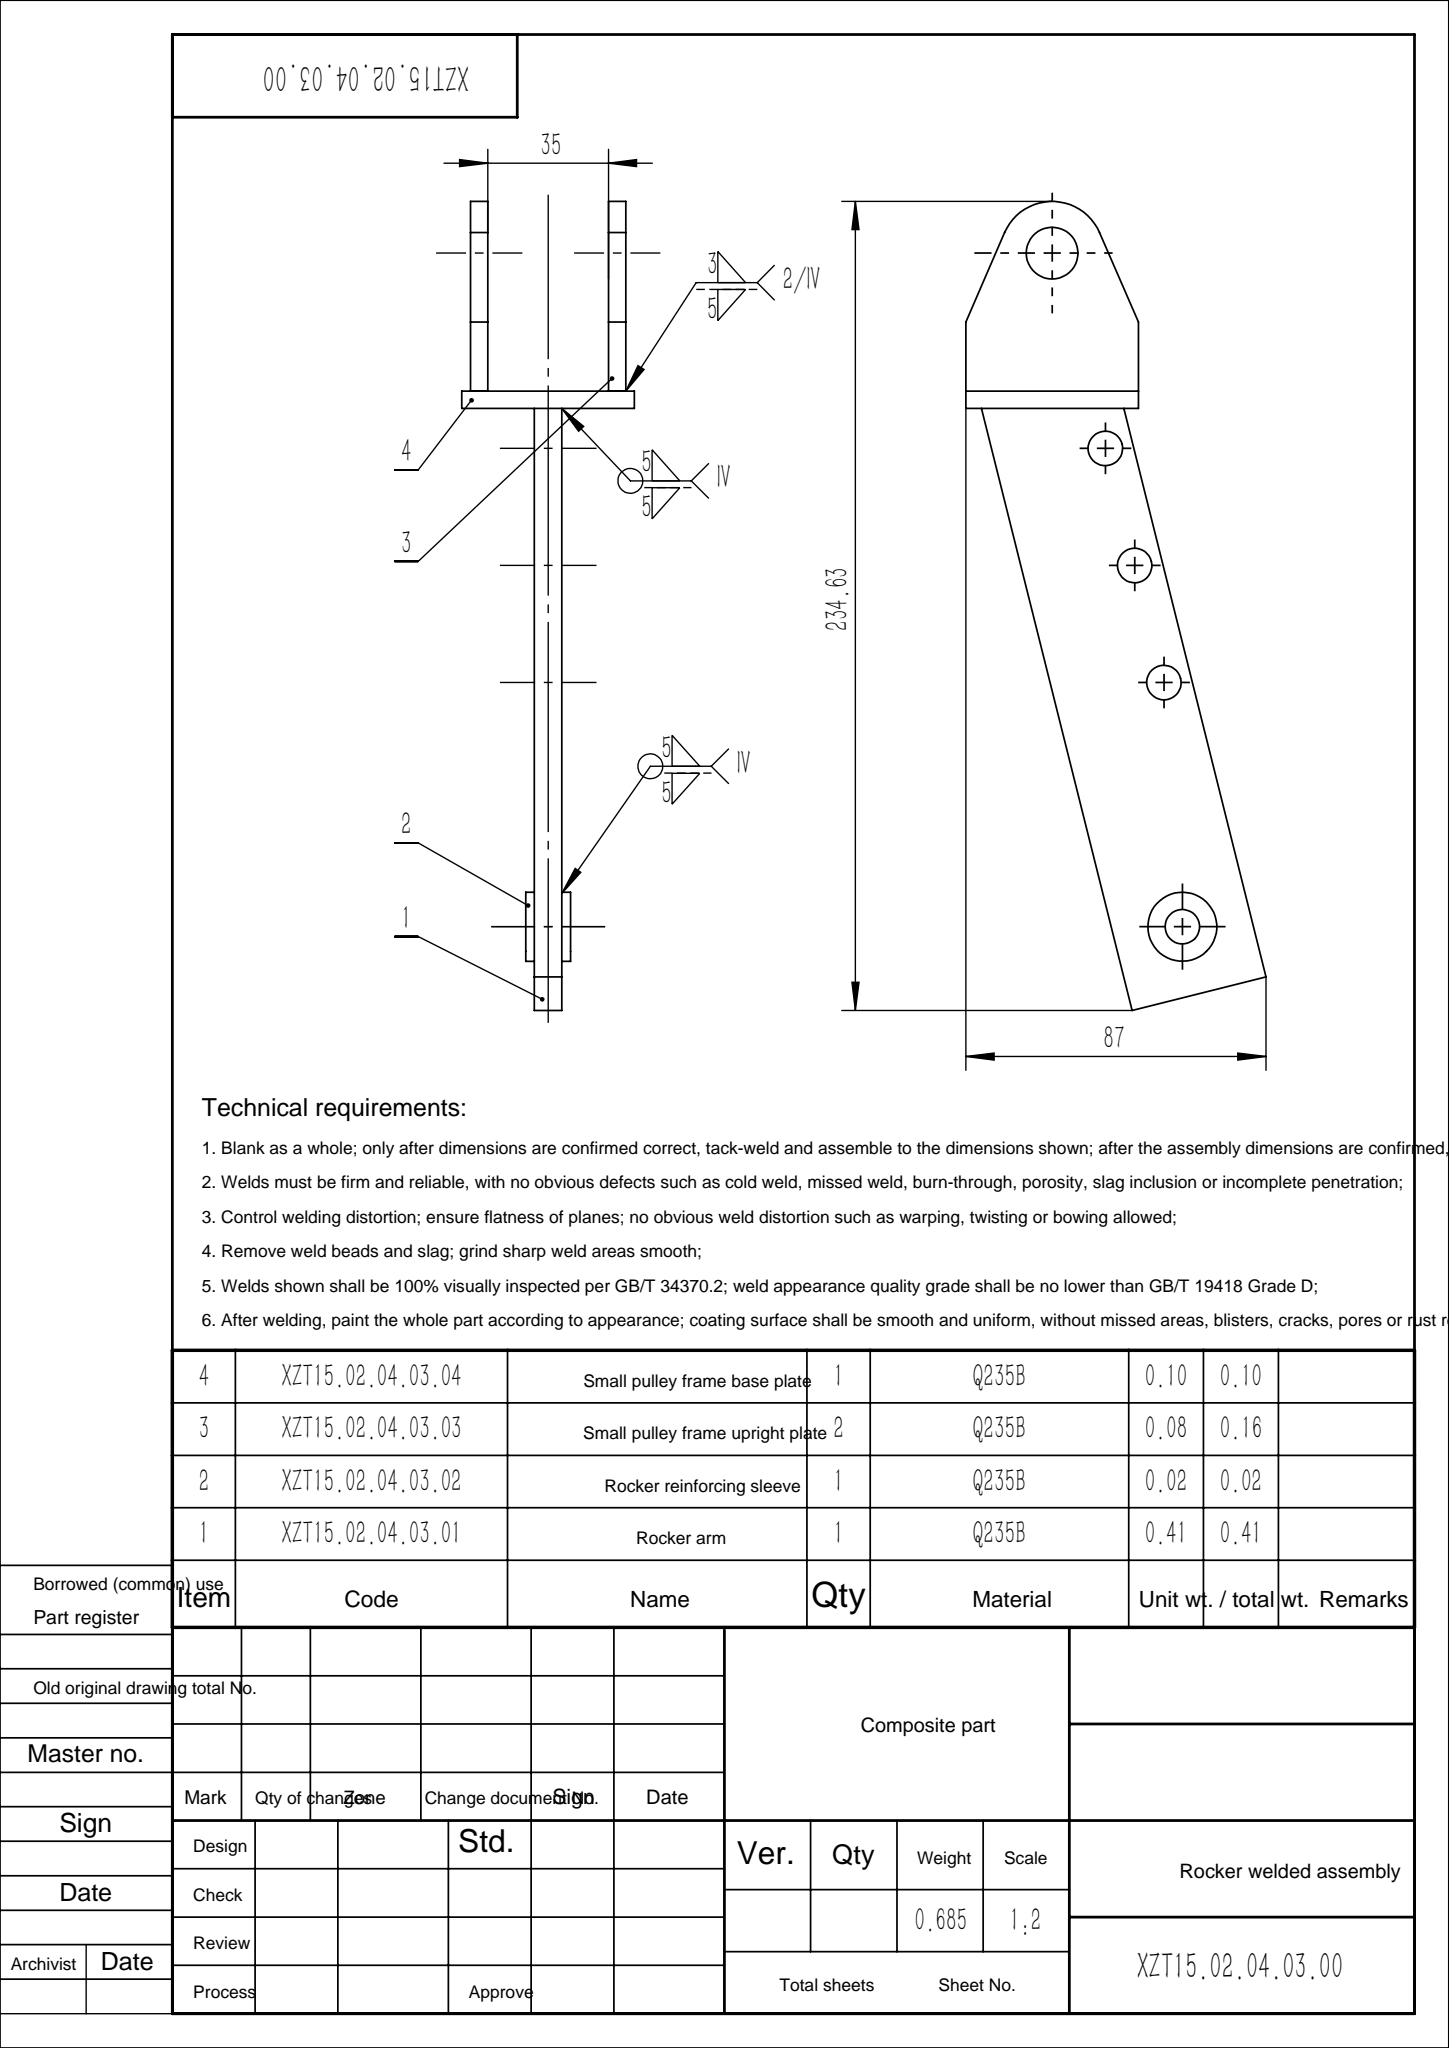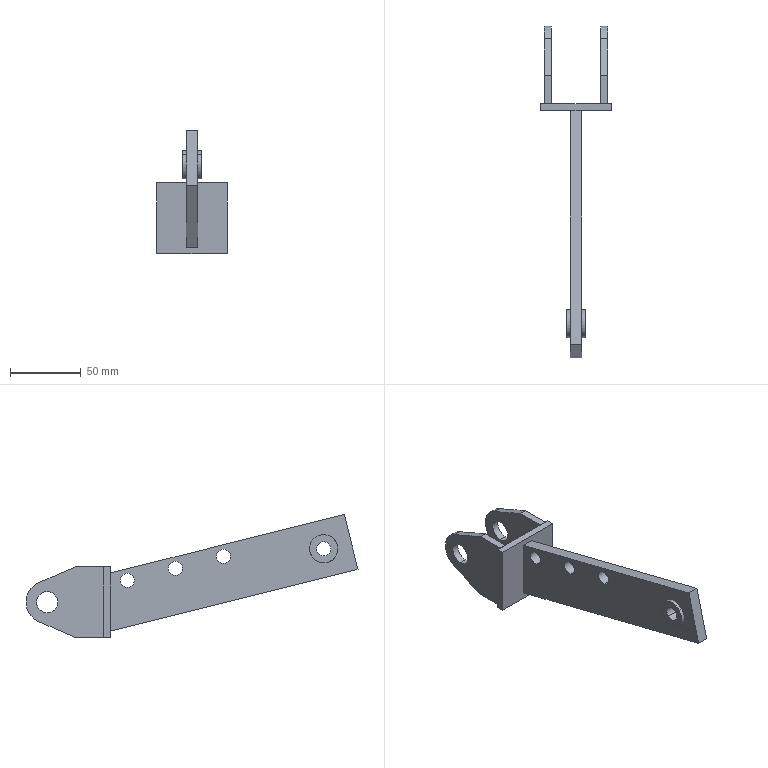Part | SolidWorks | features MirrorCompFeat 1, ReferencePattern 1 | 5 solids | 46 faces | box 50 x 234.626 x 87 mm | volume 87256 mm3 | plane 28 | cylinder 18 | commonest cylinder face diameters 10 x8 15 x4 20 x4 30 x2